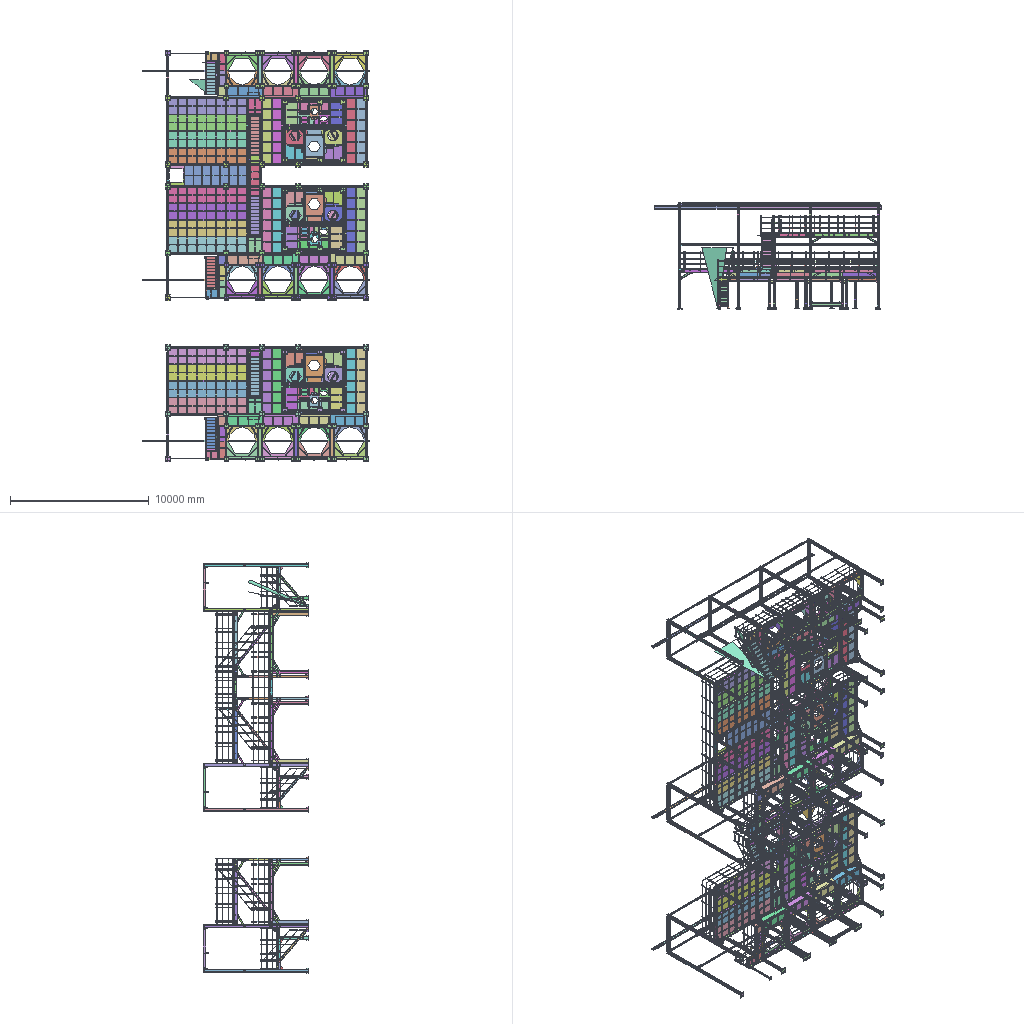Assembly | STEP file | 1060 different items | 5932 placed | box 16340 x 7600 x 29659 mm
Parts list (item | name | quantity | parent item | size | volume), first 203 of 1060 items:
1 | 粉仓立柱1主体_Default<As Machined> | x1 | in 粉仓立柱1 | 150 x 5128 x 194 mm | 19525526 mm3
2 | 立柱底Plate-400×350 | x10 | in 粉仓立柱1, 粉仓立柱2, 粉仓立柱3, 粉仓立柱4, 粉仓立柱5, 粉仓立柱6, 电柜立柱1, 电柜立柱2, 电柜立柱3, Electrical cabinet column 4 | 350 x 12 x 400 mm | 1654365 mm3
3 | 立柱Pad-400×350 | x10 | in 粉仓立柱1, 粉仓立柱2, 粉仓立柱3, 粉仓立柱4, 粉仓立柱5, 粉仓立柱6, 电柜立柱1, 电柜立柱2, 电柜立柱3, Electrical cabinet column 4 | 400 x 10 x 350 mm | 1384795 mm3
4 | 立柱底部筋Plate-200 | x32 | in 粉仓立柱1, 粉仓立柱2, 粉仓立柱3, 粉仓立柱4, 粉仓立柱5, 粉仓立柱6, 计量立柱1, 计量立柱2, 计量立柱3, 计量立柱4, 计量立柱5, 电柜立柱1, 电柜立柱2, 电柜立柱3, Electrical cabinet column 4 | 95 x 200 x 10 mm | 122000 mm3
5 | 立柱填充筋Plate-194×150 | x104 | in 粉仓立柱1, 粉仓立柱2, 粉仓立柱3, 粉仓立柱4, 粉仓立柱5, 粉仓立柱6, 计量立柱1, 计量立柱2, 计量立柱3, 计量立柱4, 电柜立柱1, 电柜立柱2, 电柜立柱3, Electrical cabinet column 4 | 72 x 10 x 176 mm | 125030 mm3
6 | 立柱腹Plate筋Plate-194×150-200 | x20 | in 粉仓立柱1, 粉仓立柱2, 粉仓立柱3, 粉仓立柱4, 粉仓立柱5, 粉仓立柱6, 计量立柱1, 计量立柱2, 计量立柱3, 计量立柱4, 电柜立柱1, 电柜立柱2, 电柜立柱3, Electrical cabinet column 4 | 230 x 180 x 10 mm | 352777 mm3
7 | 立柱翼Plate筋Plate-200 | x8 | in 粉仓立柱1, 粉仓立柱3, 粉仓立柱4, 粉仓立柱6, 电柜立柱1, 电柜立柱2, 电柜立柱3, Electrical cabinet column 4 | 155 x 150 x 10 mm | 203838 mm3
8 | 立柱填充筋Plate-194×150-1 | x2 | in 粉仓立柱1 | 72 x 10 x 176 mm | 115559 mm3
9 | 粉仓立柱2主体_Default<As Machined> | x1 | in 粉仓立柱2 | 150 x 5378 x 194 mm | 20480381 mm3
10 | 立柱腹Plate筋Plate-194×150-250 | x7 | in 粉仓立柱2, 粉仓立柱3, 粉仓立柱4, 粉仓立柱5, 粉仓立柱6 | 245 x 230 x 10 mm | 499277 mm3
11 | 立柱翼Plate筋Plate-250 | x9 | in 粉仓立柱2, 粉仓立柱3, 粉仓立柱4, 粉仓立柱5, 粉仓立柱6, 计量立柱1, 计量立柱2, 计量立柱3, 计量立柱4 | 155 x 210 x 10 mm | 296838 mm3
12 | 粉仓立柱3主体_Default<As Machined> | x1 | in 粉仓立柱3 | 150 x 5378 x 194 mm | 20474019 mm3
13 | Powder bin column 4 body_Default<As Machined> | x1 | in 粉仓立柱4 | 150 x 5378 x 194 mm | 20482501 mm3
14 | 立柱腹Plate筋Plate-194×150-12 | x10 | in 粉仓立柱4, 粉仓立柱5, 粉仓立柱6, 电柜立柱1, 电柜立柱2 | 200 x 100 x 8 mm | 126933 mm3
15 | Powder bin column 5 body_Default<As Machined> | x1 | in 粉仓立柱5 | 150 x 7578 x 194 mm | 28858083 mm3
16 | 立柱翼Plate筋Plate-150 | x4 | in 粉仓立柱5, 粉仓立柱6, 电柜立柱1, 电柜立柱2 | 154 x 154 x 10 mm | 217969 mm3
17 | 粉仓立柱6主体_Default<As Machined> | x1 | in 粉仓立柱6 | 150 x 7578 x 194 mm | 28847525 mm3
18 | 粉仓主梁1主体_Default<As Machined> | x1 | in 粉仓主梁1 | 4730 x 250 x 295 mm | 19829494 mm3
19 | Beam填充筋Plate-250×125 | x23 | in 粉仓主梁1, 粉仓主梁2, 粉仓主梁4, 粉仓主梁5, Powder bin main beam 7, 粉仓主梁8, 粉仓主梁9, 粉仓主梁11, 计量主梁1, 计量主梁2, 计量主梁5, 计量主梁6 | 55 x 10 x 232 mm | 126600 mm3
20 | 筋Plate-250×125-250 | x13 | in 粉仓主梁1, 粉仓主梁2, 粉仓主梁4, 粉仓主梁5, 粉仓主梁6, Powder bin main beam 7, 粉仓主梁11, 计量主梁1, 计量主梁2 | 215 x 232 x 10 mm | 429336 mm3
21 | 护栏连接Plate-250×125 | x29 | in 粉仓主梁1, 粉仓主梁2, 粉仓主梁3, 粉仓主梁4, Powder bin main beam 7, 粉仓主梁11 | 40 x 232 x 6 mm | 52883 mm3
22 | 筋Plate-250×125-200 | x10 | in 粉仓主梁1, 粉仓主梁5, 粉仓主梁6, Powder bin main beam 7, 粉仓主梁8, 粉仓主梁9, 粉仓主梁11, 计量主梁5 | 217 x 232 x 10 mm | 354786 mm3
23 | 筋Plate-250×125-150 | x30 | in 粉仓主梁1, 粉仓主梁2, 粉仓主梁3, 粉仓主梁4, 粉仓主梁5, 粉仓主梁6, 粉仓主梁8, 粉仓主梁9, 粉仓主梁10, 粉仓主梁11, 计量主梁1, 计量主梁2, 计量主梁6 | 190 x 232 x 10 mm | 269336 mm3
24 | 粉仓主梁2主体_Default<As Machined> | x1 | in 粉仓主梁2 | 4730 x 250 x 125 mm | 17453380 mm3
25 | 粉仓主梁3主体_Default<As Machined> | x1 | in 粉仓主梁3 | 2430 x 250 x 125 mm | 8963145 mm3
26 | 粉仓主梁4主体_Default<As Machined> | x1 | in 粉仓主梁4 | 4620 x 250 x 125 mm | 17048565 mm3
27 | 筋Plate-250×125-100 | x10 | in 粉仓主梁4, 粉仓主梁5, Powder bin main beam 7, 计量主梁1, 计量主梁2 | 185 x 232 x 8 mm | 168205 mm3
28 | Powder bin main beam 5 body_Default<As Machined> | x1 | in 粉仓主梁5 | 4586 x 250 x 125 mm | 16921020 mm3
29 | 筋Plate-250×125-150-30度 | x2 | in 粉仓主梁5, 粉仓主梁6 | 250 x 232 x 10 mm | 378866 mm3
30 | 筋Plate-250×125-200-30度 | x4 | in 粉仓主梁5, 粉仓主梁6, Powder bin main beam 7 | 265 x 232 x 10 mm | 450796 mm3
31 | 粉仓主梁6主体_Default<As Machined> | x1 | in 粉仓主梁6 | 4655 x 250 x 125 mm | 17188833 mm3
32 | 粉仓主梁7主体_Default<As Machined> | x1 | in Powder bin main beam 7 | 4586 x 250 x 125 mm | 16921020 mm3
33 | 粉仓主梁8主体_Default<As Machined> | x1 | in 粉仓主梁8 | 2455 x 250 x 125 mm | 9055569 mm3
34 | 筋Plate-250×125-200-60度 | x6 | in 粉仓主梁8, 粉仓主梁9, 粉仓主梁10 | 225 x 232 x 10 mm | 372036 mm3
35 | 粉仓主梁9主体_Default<As Machined> | x1 | in 粉仓主梁9 | 2655 x 250 x 125 mm | 9794957 mm3
36 | 粉仓主梁10主体_Default<As Machined> | x1 | in 粉仓主梁10 | 1955 x 250 x 125 mm | 7207100 mm3
37 | Powder bin main beam 11 body_Default<As Machined> | x1 | in 粉仓主梁11 | 3440 x 250 x 125 mm | 12683851 mm3
38 | 粉仓楼梯支撑Plate | x2 | in 粉仓主梁11 | 120 x 232 x 10 mm | 268929 mm3
39 | 护栏连接Plate-250×125-1 | x1 | in 粉仓主梁11 | 40 x 184 x 59.5 mm | 52864 mm3
40 | 粉仓主梁12主体_Default<As Machined> | x1 | in 粉仓主梁12 | 1815 x 200 x 360 mm | 5338714 mm3
41 | Beam填充筋Plate-200×100 | x7 | in 粉仓主梁12, 粉仓主梁13, 粉仓主梁14, 休息台主梁1, 休息台主梁2, 休息台主梁4, 休息台主梁5 | 8 x 184 x 37.25 mm | 54032 mm3
42 | 粉仓主梁13主体_Default<As Machined> | x1 | in 粉仓主梁13 | 2255 x 200 x 100 mm | 5995232 mm3
43 | 筋Plate-200×100-200 | x7 | in 粉仓主梁13, 休息台主梁1, 休息台主梁2, 休息台主梁4, 休息台主梁5, 计量主梁3 | 202 x 184 x 10 mm | 304236 mm3
44 | 筋Plate-200×100-150 | x16 | in 粉仓主梁13, 粉仓主梁15, 计量主梁4, 计量主梁7, 计量主梁8, 电柜主梁1, 电柜主梁3, 电柜主梁6 | 182 x 184 x 10 mm | 220956 mm3
45 | 筋Plate-200×100-200-30度 | x2 | in 粉仓主梁13, 粉仓主梁15 | 245 x 184 x 10 mm | 379966 mm3
46 | 粉仓主梁14主体_Default<As Machined> | x1 | in 粉仓主梁14 | 1955 x 200 x 360 mm | 5712085 mm3
47 | 粉仓主梁15主体_Default<As Machined> | x1 | in 粉仓主梁15 | 2255 x 200 x 100 mm | 5995232 mm3
48 | 粉仓辅梁1_Default<As Machined> | x1 | in 125Z正极线_粉仓Flat(E1) | 520 x 150 x 75 mm | 916827 mm3
49 | Powder bin secondary beam 2_Default<As Machined> | x1 | in 125Z正极线_粉仓Flat(E1) | 365 x 150 x 75 mm | 640161 mm3
50 | 粉仓辅梁3主体_Default<As Machined> | x2 | in 粉仓辅梁3 | 775 x 100 x 50 mm | 912656 mm3
51 | 粉仓辅梁4主体_Default<As Machined> | x1 | in 粉仓辅梁4 | 75 x 150 x 310 mm | 510249 mm3
52 | 粉仓辅梁5_Default<As Machined> | x1 | in 125Z正极线_粉仓Flat(E1) | 440 x 150 x 75 mm | 774032 mm3
53 | Powder bin secondary beam 6 body_Default<As Machined> | x1 | in 粉仓辅梁6 | 1245 x 150 x 350 mm | 2721156 mm3
54 | 粉仓辅梁7主体_Default<As Machined> | x1 | in 粉仓辅梁7 | 1545 x 150 x 280 mm | 3131691 mm3
55 | 粉仓辅梁8_Default<As Machined> | x1 | in 125Z正极线_粉仓Flat(E1) | 440 x 150 x 75 mm | 774032 mm3
56 | Powder bin secondary beam 9 body_Default<As Machined> | x1 | in 粉仓辅梁9 | 1445 x 150 x 75 mm | 2567894 mm3
57 | 筋Plate-150×75-150 | x18 | in 粉仓辅梁9, 粉仓辅梁10, 粉仓辅梁11, 粉仓辅梁13, 粉仓辅梁14, Powder bin secondary beam 16, 粉仓辅梁18, Metering secondary beam 5, Metering secondary beam 7, 计量辅梁15, Metering secondary beam 16 | 165 x 136 x 10 mm | 178316 mm3
58 | 筋Plate-150×75-150-60度 | x6 | in 粉仓辅梁9, 粉仓辅梁11, 粉仓辅梁14 | 175 x 136 x 10 mm | 189716 mm3
59 | 粉仓辅梁10主体_Default<As Machined> | x1 | in 粉仓辅梁10 | 2255 x 150 x 75 mm | 4013694 mm3
60 | 筋Plate-150×75-100 | x12 | in 粉仓辅梁10, 粉仓辅梁13, 粉仓辅梁18, 计量辅梁1, Metering secondary beam 5, 计量辅梁12, Metering secondary beam 16 | 165 x 136 x 8 mm | 100309 mm3
61 | 筋Plate-150×75-150-30度 | x4 | in 粉仓辅梁10, 粉仓辅梁13, Powder bin secondary beam 16, 粉仓辅梁18 | 200 x 136 x 10 mm | 222316 mm3
62 | 粉仓辅梁11主体_Default<As Machined> | x1 | in 粉仓辅梁11 | 1545 x 150 x 75 mm | 2746388 mm3
63 | 粉仓辅梁12_Default<As Machined> | x1 | in 125Z正极线_粉仓Flat(E1) | 430 x 150 x 75 mm | 756182 mm3
64 | 粉仓辅梁13主体_Default<As Machined> | x1 | in 粉仓辅梁13 | 2255 x 150 x 75 mm | 4013694 mm3
65 | 粉仓辅梁14主体_Default<As Machined> | x1 | in 粉仓辅梁14 | 1245 x 150 x 75 mm | 2210907 mm3
66 | 粉仓辅梁15主体_Default<As Machined> | x2 | in 粉仓辅梁15 | 915 x 100 x 50 mm | 1078548 mm3
67 | 粉仓辅梁16主体_Default<As Machined> | x1 | in Powder bin secondary beam 16 | 2255 x 150 x 230 mm | 4605807 mm3
68 | Powder bin secondary beam 17 body_Default<As Machined> | x2 | in 粉仓辅梁17 | 615 x 100 x 50 mm | 723066 mm3
69 | 粉仓辅梁18主体_Default<As Machined> | x1 | in 粉仓辅梁18 | 2255 x 150 x 75 mm | 4013694 mm3
70 | Powder bin diagonal beam 1_Default<As Machined> | x1 | in 125Z正极线_粉仓Flat(E1) | 502.735 x 200 x 870.763 mm | 2354862 mm3
71 | 粉仓Diagonal Brace梁2_Default<As Machined> | x1 | in 125Z正极线_粉仓Flat(E1) | 957.365 x 200 x 552.735 mm | 2621556 mm3
72 | 粉仓Diagonal Brace梁3-2_Default<As Machined> | x1 | in 125Z正极线_粉仓Flat(E1) | 253.301 x 150 x 438.731 mm | 738333 mm3
73 | 粉仓Diagonal Brace梁3-1_Default<As Machined> | x1 | in 125Z正极线_粉仓Flat(E1) | 273.301 x 150 x 473.372 mm | 809730 mm3
74 | 粉仓Diagonal Brace梁4_Default<As Machined> | x1 | in 125Z正极线_粉仓Flat(E1) | 473.372 x 150 x 273.301 mm | 809730 mm3
75 | Powder bin diagonal beam 5_Default<As Machined> | x1 | in 125Z正极线_粉仓Flat(E1) | 453.301 x 150 x 785.141 mm | 1452308 mm3
76 | 粉仓Diagonal Brace梁6-1_Default<As Machined> | x1 | in 125Z正极线_粉仓Flat(E1) | 525.333 x 150 x 303.301 mm | 916827 mm3
77 | 粉仓Diagonal Brace梁6-2_Default<As Machined> | x1 | in 125Z正极线_粉仓Flat(E1) | 646.577 x 150 x 373.301 mm | 1166718 mm3
78 | 粉仓Diagonal Brace梁7_Default<As Machined> | x1 | in 125Z正极线_粉仓Flat(E1) | 462.735 x 200 x 801.481 mm | 2141507 mm3
79 | 粉仓Diagonal Brace梁8_Default<As Machined> | x1 | in 125Z正极线_粉仓Flat(E1) | 671.577 x 200 x 387.735 mm | 1741466 mm3
80 | 粉仓Diagonal Brace梁9_Default<As Machined> | x1 | in 125Z正极线_粉仓Flat(E1) | 522.735 x 200 x 905.404 mm | 2461540 mm3
81 | 粉仓Diagonal Brace梁10_Default<As Machined> | x1 | in 125Z正极线_粉仓Flat(E1) | 1148 x 200 x 662.735 mm | 3208282 mm3
82 | 粉仓花纹Plate | x1 | in 125Z正极线_粉仓Flat(E1) | 7625 x 4925 x 3 mm | 81712704 mm3
83 | 休息台主梁1主体_Default<As Machined> | x1 | in 休息台主梁1 | 2430 x 200 x 200 mm | 6806772 mm3
84 | 筋Plate-200×100-5 | x34 | in 休息台主梁1, 休息台主梁2, 休息台主梁4, 休息台主梁5, Landing main beam 6, 计量主梁7, 计量主梁8, 电柜主梁2, 电柜主梁5, 电柜主梁8, 粉仓楼梯通道主梁1, 粉仓楼梯通道主梁2, 电柜通道主梁1 | 120 x 184 x 6 mm | 69909 mm3
85 | 护栏连接Plate-200×100 | x49 | in 休息台主梁1, 休息台主梁2, 休息台主梁3, 休息台主梁4, 休息台主梁5, Landing main beam 6, 电柜主梁2, 电柜主梁3, 电柜主梁4, 电柜主梁8, 粉仓楼梯通道主梁1, 粉仓楼梯通道主梁2, 电柜通道主梁1, Electrical cabinet walkway main beam 2 | 40 x 184 x 6 mm | 41363 mm3
86 | 休息台主梁2主体_Default<As Machined> | x1 | in 休息台主梁2 | 4730 x 200 x 200 mm | 13901578 mm3
87 | 休息台主梁3主体_Default<As Machined> | x1 | in 休息台主梁3 | 4586 x 200 x 100 mm | 12200555 mm3
88 | 筋Plate-200×100-100 | x50 | in 休息台主梁3, Landing main beam 6, Landing main beam 7, 休息台主梁8, 计量主梁3, 电柜主梁1, 电柜主梁3, 电柜主梁4, 电柜主梁6, 电柜主梁7, 电柜主梁9 | 182 x 184 x 8 mm | 124941 mm3
89 | Landing main beam 4 body_Default<As Machined> | x1 | in 休息台主梁4 | 4730 x 200 x 200 mm | 13878197 mm3
90 | 休息台主梁5主体_Default<As Machined> | x1 | in 休息台主梁5 | 2430 x 200 x 200 mm | 6806772 mm3
91 | 休息台主梁6主体_Default<As Machined> | x1 | in Landing main beam 6 | 4586 x 200 x 100 mm | 12200555 mm3
92 | 筋Plate-200×100-194 | x2 | in Landing main beam 6, 电柜主梁8 | 202 x 184 x 10 mm | 304236 mm3
93 | 休息台主梁7主体_Default<As Machined> | x1 | in Landing main beam 7 | 4680 x 200 x 100 mm | 12462557 mm3
94 | Landing main beam 8 body_Default<As Machined> | x1 | in 休息台主梁8 | 4680 x 200 x 100 mm | 12462557 mm3
95 | 休息台辅梁1主体_Default<As Machined> | x10 | in Landing secondary beam 1 | 1350 x 100 x 50 mm | 1593996 mm3
96 | 筋Plate-100×50-5 | x91 | in Landing secondary beam 1, 计量辅梁3, 计量辅梁11, 电柜辅梁1, 电柜辅梁3, 电柜通道辅梁1 | 95 x 86 x 6 mm | 27288 mm3
97 | 休息台角钢1_Default<As Machined> | x12 | in 125Z正极线_粉仓Flat(E1) | 721.5 x 50 x 50 mm | 278924 mm3
98 | 休息台花纹Plate 1 | x1 | in 125Z正极线_粉仓Flat(E1) | 1620 x 4900 x 3 mm | 23686830 mm3
99 | 休息台花纹Plate 2 | x1 | in 125Z正极线_粉仓Flat(E1) | 1620 x 4900 x 3 mm | 23500005 mm3
100 | 休息台花纹Plate 3 | x1 | in 125Z正极线_粉仓Flat(E1) | 4350 x 248 x 3 mm | 3156330 mm3
101 | 休息台花纹Plate 4 | x1 | in 125Z正极线_粉仓Flat(E1) | 4350 x 248 x 3 mm | 3156330 mm3
102 | Powder bin stair body_Default<As Machined> | x1 | in 粉仓楼梯 | 800 x 2588 x 3603 mm | 21206724 mm3
103 | 粉仓楼梯踏Plate 1 | x12 | in 粉仓楼梯 | 248 x 100 x 674 mm | 693251 mm3
104 | Stair base plate 2-1 | x2 | in 粉仓楼梯 | 120 x 160 x 12 mm | 218038 mm3
105 | 楼梯踏Plate 3 | x1 | in 粉仓楼梯 | 686 x 50 x 860 mm | 1690832 mm3
106 | Powder bin stair closing plate 1 | x12 | in 粉仓楼梯 | 674 x 3 x 100 mm | 202200 mm3
107 | 粉仓楼梯封Plate 2 | x1 | in 粉仓楼梯 | 674 x 3 x 138 mm | 279036 mm3
108 | 粉仓楼梯护栏1主体_Default<As Machined> | x2 | in 粉仓楼梯护栏1, 粉仓楼梯护栏2 | 25 x 3380 x 2914 mm | 1521542 mm3
109 | 楼梯护栏连接Plate 1 | x22 | in 粉仓楼梯护栏1, 粉仓楼梯护栏2, 中转釜楼梯护栏1, 中转釜楼梯护栏2 | 125 x 8 x 42 mm | 38206 mm3
110 | 粉仓护栏FixedPlate 1 | x2 | in 粉仓楼梯护栏2 | 85 x 40 x 40 mm | 13802 mm3
111 | Stair connecting plate 1 | x4 | in 粉仓楼梯, Transfer kettle stair | - | 160302 mm3
112 | 粉仓楼梯护栏连接Plate | x1 | in 粉仓楼梯 | 40 x 190.865 x 6 mm | 38885 mm3
113 | 粉仓护栏FixedPlate 2 | x2 | in 粉仓楼梯 | 45 x 40 x 63 mm | 11762 mm3
114 | 粉仓楼梯支承梁主体-194×150_Default<As Machined> | x1 | in 粉仓楼梯支承梁 | 940 x 150 x 194 mm | 3552325 mm3
115 | 筋Plate-194×150-100 | x1 | in 粉仓楼梯支承梁 | 200 x 176 x 8 mm | 160789 mm3
116 | 护栏90度栏杆_Default<As Machined> | x6 | in 护栏90度 | 397.5 x 25 x 397.5 mm | 82894 mm3
117 | 护栏90度立柱主体_Default<As Machined> | x4 | in 护栏90度立柱 | 40 x 1500 x 40 mm | 436819 mm3
118 | 40方管堵头 | x212 | in 护栏90度立柱, Powder bin guardrail 1 column, 护栏立柱2, 粉仓护栏2-1立柱, 粉仓护栏3-1立柱, 粉仓护栏3-2立柱, 粉仓护栏5立柱, 粉仓护栏立柱6, 粉仓护栏6-1立柱, 护栏立柱1, 粉仓护栏8-1立柱, 粉仓护栏8-2立柱, 粉仓护栏9立柱, Powder bin guardrail 9-1 column, 电柜护栏2立柱, 电柜护栏4立柱, 中转釜护栏2立柱, 中转釜护栏3立柱, 中转釜护栏4立柱, 中转釜护栏5立柱, 中转釜护栏7-1立柱, 中转釜护栏立柱7-2, Guardrail column 8-1, Guardrail column 8-2, Powder bin stair walkway guardrail 1 column, 粉仓楼梯通道护栏立柱2-1, 电柜通道护栏1立柱 | 40 x 18.9 x 40 mm | 8663 mm3
119 | 护栏90度踢脚Plate-1 | x2 | in 护栏90度 | 410 x 100 x 20 mm | 90870 mm3
120 | 护栏90度踢脚Plate-2 | x2 | in 护栏90度 | 410 x 100 x 20 mm | 119752 mm3
121 | 粉仓护栏1立柱主体_Default<As Machined> | x1 | in Powder bin guardrail 1 column | 40 x 1500 x 40 mm | 436819 mm3
122 | 护栏立柱2主体_Default<As Machined> | x60 | in 护栏立柱2 | 40 x 1500 x 40 mm | 432313 mm3
123 | 粉仓踢脚Plate 1 | x1 | in 粉仓护栏1 | 4345 x 100 x 20 mm | 998785 mm3
124 | 粉仓护栏栏杆1_Default<As Machined> | x1 | in 粉仓护栏1 | 4305 x 825 x 25 mm | 1430222 mm3
125 | 粉仓护栏2-1立柱主体_Default<As Machined> | x2 | in 粉仓护栏2-1立柱 | 40 x 1500 x 40 mm | 436819 mm3
126 | 粉仓踢脚Plate 2 | x1 | in 粉仓护栏2 | 3814 x 100 x 20 mm | 876724 mm3
127 | 粉仓护栏栏杆2_Default<As Machined> | x3 | in 粉仓护栏2 | 3734 x 25 x 25 mm | 413507 mm3
128 | Powder bin guardrail 3-1 column body_Default<As Machined> | x1 | in 粉仓护栏3-1立柱 | 40 x 1500 x 40 mm | 436819 mm3
129 | Powder bin toe plate 3 | x1 | in 粉仓护栏3 | 3694 x 100 x 20 mm | 849140 mm3
130 | 粉仓护栏栏杆3_Default<As Machined> | x1 | in 粉仓护栏3 | 3614 x 825 x 25 mm | 1200655 mm3
131 | 粉仓护栏3-2立柱主体_Default<As Machined> | x1 | in 粉仓护栏3-2立柱 | 40 x 1500 x 40 mm | 436531 mm3
132 | Powder bin toe plate 4 | x2 | in 粉仓护栏4 | 2430 x 100 x 20 mm | 558584 mm3
133 | 粉仓护栏栏杆4_Default<As Machined> | x2 | in 粉仓护栏4 | 2430 x 825 x 25 mm | 807303 mm3
134 | 粉仓踢脚Plate 5 | x1 | in 粉仓护栏5 | 2168 x 100 x 20 mm | 498243 mm3
135 | Powder bin guardrail rail 5_Default<As Machined> | x1 | in 粉仓护栏5 | 2128 x 825 x 25 mm | 706805 mm3
136 | 粉仓护栏5立柱主体_Default<As Machined> | x1 | in 粉仓护栏5立柱 | 40 x 1500 x 40 mm | 436819 mm3
137 | 粉仓踢脚Plate 6 | x1 | in 粉仓护栏6 | 2290 x 100 x 20 mm | 526402 mm3
138 | 粉仓护栏栏杆6_Default<As Machined> | x1 | in 粉仓护栏6 | 2250 x 825 x 25 mm | 747503 mm3
139 | 粉仓护栏6立柱主体_Default<As Machined> | x1 | in 粉仓护栏立柱6 | 40 x 1500 x 40 mm | 436819 mm3
140 | 粉仓踢脚Plate 6-1 | x1 | in 粉仓护栏6-1 | 2290 x 100 x 20 mm | 526402 mm3
141 | Powder bin guardrail rail 6-1_Default<As Machined> | x1 | in 粉仓护栏6-1 | 2250 x 825 x 25 mm | 747503 mm3
142 | 粉仓护栏6-1立柱主体_Default<As Machined> | x1 | in 粉仓护栏6-1立柱 | 40 x 1500 x 40 mm | 436819 mm3
143 | 护栏立柱1主体_Default<As Machined> | x9 | in 护栏立柱1 | 40 x 1500 x 40 mm | 438684 mm3
144 | Powder bin toe plate 7 | x1 | in Powder bin guardrail 7 | 3390 x 100 x 20 mm | 779259 mm3
145 | 粉仓护栏栏杆7_Default<As Machined> | x1 | in Powder bin guardrail 7 | 3350 x 825 x 25 mm | 1112948 mm3
146 | Powder bin guardrail 8-1 column body_Default<As Machined> | x1 | in 粉仓护栏8-1立柱 | 40 x 1500 x 40 mm | 436819 mm3
147 | 粉仓踢脚Plate 8 | x1 | in 粉仓护栏8 | 3330 x 100 x 20 mm | 765467 mm3
148 | 粉仓护栏栏杆8_Default<As Machined> | x3 | in 粉仓护栏8 | 3275 x 25 x 25 mm | 362677 mm3
149 | Powder bin guardrail 8-2 column body_Default<As Machined> | x1 | in 粉仓护栏8-2立柱 | 40 x 1500 x 40 mm | 436819 mm3
150 | 粉仓护栏9立柱主体_Default<As Machined> | x3 | in 粉仓护栏9立柱 | 40 x 1500 x 40 mm | 436819 mm3
151 | 粉仓踢脚Plate 9 | x3 | in 粉仓护栏9 | 2365 x 100 x 20 mm | 543643 mm3
152 | 粉仓护栏栏杆9_Default<As Machined> | x3 | in 粉仓护栏9 | 2325 x 825 x 25 mm | 772419 mm3
153 | 粉仓护栏9-1立柱主体_Default<As Machined> | x3 | in Powder bin guardrail 9-1 column | 40 x 1500 x 40 mm | 436819 mm3
154 | 粉仓踢脚Plate 9-1 | x3 | in 粉仓护栏9-1 | 2365 x 100 x 20 mm | 543643 mm3
155 | 粉仓护栏栏杆9-1_Default<As Machined> | x3 | in 粉仓护栏9-1 | 2325 x 825 x 25 mm | 772419 mm3
156 | Diagonal Brace矩形管-100×50-45度_Default<As Machined> | x1 | in Diagonal BraceComponent-45度 | 721.249 x 721.249 x 50 mm | 994577 mm3
157 | Diagonal Brace连接Plate-45度 | x2 | in Diagonal BraceComponent-45度 | 280 x 10 x 120 mm | 322431 mm3
158 | Diagonal Brace矩形管-60度_Default<As Machined> | x30 | in Diagonal BraceComponent-60度 | 823.131 x 475.235 x 50 mm | 902687 mm3
159 | Diagonal Brace连接Plate 1-1 | x30 | in Diagonal BraceComponent-60度 | 280 x 10 x 120 mm | 322431 mm3
160 | Diagonal Brace连接Plate 2-2 | x30 | in Diagonal BraceComponent-60度 | 360 x 10 x 100 mm | 346431 mm3
161 | 立柱底Plate-400×350-1 | x6 | in 计量立柱1, 计量立柱2, 计量立柱3, 计量立柱4, 计量立柱5 | - | -
162 | 立柱Pad-400×350-1 | x6 | in 计量立柱1, 计量立柱2, 计量立柱3, 计量立柱4, 计量立柱5 | 400 x 10 x 350 mm | 1384795 mm3
163 | 计量立柱1主体_Default<As Machined> | x1 | in 计量立柱1 | 150 x 2778 x 194 mm | 10580424 mm3
164 | Metering column 2 body_Default<As Machined> | x1 | in 计量立柱2 | 150 x 2778 x 194 mm | 10580424 mm3
165 | 计量立柱3主体_Default<As Machined> | x1 | in 计量立柱3 | 150 x 2778 x 194 mm | 10580424 mm3
166 | 计量立柱4主体_Default<As Machined> | x1 | in 计量立柱4 | 150 x 2778 x 194 mm | 10580424 mm3
167 | Metering column 5 body_Default<As Machined> | x2 | in 计量立柱5 | 150 x 2578 x 194 mm | 9824598 mm3
168 | 立柱填充筋Plate-194×150-2 | x4 | in 计量立柱5 | 72 x 10 x 176 mm | 115559 mm3
169 | 计量主梁1主体_Default<As Machined> | x1 | in 计量主梁1 | 3986 x 250 x 125 mm | 14702858 mm3
170 | 筋Plate-250×125-150-45度 | x6 | in 计量主梁1, 计量主梁2, 计量主梁5 | 215 x 232 x 10 mm | 315156 mm3
171 | 计量主梁2主体_Default<As Machined> | x1 | in 计量主梁2 | 3986 x 250 x 125 mm | 14702858 mm3
172 | 计量主梁3主体_Default<As Machined> | x1 | in 计量主梁3 | 4030 x 200 x 100 mm | 10713895 mm3
173 | Beam填充筋Plate-200×100-2 | x4 | in 计量主梁3, 计量主梁4 | 45 x 10 x 184 mm | 81800 mm3
174 | 计量主梁主4体_Default<As Machined> | x1 | in 计量主梁4 | 4030 x 200 x 100 mm | 10713895 mm3
175 | 计量主梁5主体_Default<As Machined> | x1 | in 计量主梁5 | 4055 x 250 x 125 mm | 14970670 mm3
176 | 计量主梁6主体_Default<As Machined> | x1 | in 计量主梁6 | 4055 x 250 x 125 mm | 14970670 mm3
177 | 筋Plate-250×125-5 | x1 | in 计量主梁6 | 135 x 232 x 6 mm | 105651 mm3
178 | 计量主梁7主体_Default<As Machined> | x1 | in 计量主梁7 | 2170 x 200 x 100 mm | 5768543 mm3
179 | 筋Plate-200×100-150 -45度 | x2 | in 计量主梁7, 计量主梁8 | 196 x 184 x 10 mm | 240506 mm3
180 | 计量主梁8主体_Default<As Machined> | x1 | in 计量主梁8 | 2170 x 200 x 100 mm | 5768543 mm3
181 | 计量辅梁1主体_Default<As Machined> | x1 | in 计量辅梁1 | 1268 x 150 x 75 mm | 2251068 mm3
182 | 计量辅梁2_Default<As Machined> | x1 | in 125Z正极线_计量Flat(E1) | 1280 x 150 x 75 mm | 2273380 mm3
183 | Metering secondary beam 3 body_Default<As Machined> | x1 | in 计量辅梁3 | 1015 x 100 x 50 mm | 1197042 mm3
184 | Metering secondary beam 4 body_Default<As Machined> | x1 | in 计量辅梁4 | 1280 x 150 x 75 mm | 2273380 mm3
185 | 计量辅梁5主体_Default<As Machined> | x1 | in Metering secondary beam 5 | 1540 x 150 x 75 mm | 2737463 mm3
186 | 筋Plate-150×75-5 | x17 | in Metering secondary beam 5, Metering secondary beam 7, 计量辅梁8, 计量辅梁15, Metering secondary beam 16, 电柜辅梁2 | 110 x 136 x 6 mm | 47835 mm3
187 | Metering secondary beam 6_Default<As Machined> | x1 | in 125Z正极线_计量Flat(E1) | 605 x 150 x 75 mm | 1068546 mm3
188 | 计量辅梁7主体_Default<As Machined> | x1 | in Metering secondary beam 7 | 1540 x 150 x 75 mm | 2737463 mm3
189 | 计量辅梁8主体_Default<As Machined> | x1 | in 计量辅梁8 | 600 x 150 x 75 mm | 1059622 mm3
190 | 计量辅梁9_Default<As Machined> | x1 | in 125Z正极线_计量Flat(E1) | 600 x 150 x 75 mm | 1059622 mm3
191 | 计量辅梁10主体_Default<As Machined> | x2 | in 计量辅梁10 | 932.5 x 100 x 50 mm | 1099284 mm3
192 | 计量辅梁11主体_Default<As Machined> | x1 | in 计量辅梁11 | 1015 x 100 x 50 mm | 1197042 mm3
193 | 计量辅梁12主体_Default<As Machined> | x1 | in 计量辅梁12 | 1268 x 150 x 75 mm | 2251068 mm3
194 | 计量辅梁13主体_Default<As Machined> | x2 | in 计量辅梁13 | 932.5 x 100 x 50 mm | 1099284 mm3
195 | 计量辅梁14_Default<As Machined> | x1 | in 125Z正极线_计量Flat(E1) | 605 x 150 x 75 mm | 1068546 mm3
196 | 计量辅梁15主体_Default<As Machined> | x1 | in 计量辅梁15 | 1540 x 150 x 75 mm | 2737463 mm3
197 | 计量辅梁16主体_Default<As Machined> | x1 | in Metering secondary beam 16 | 1540 x 150 x 75 mm | 2737463 mm3
198 | 计量Diagonal Brace梁1_Default<As Machined> | x1 | in 125Z正极线_计量Flat(E1) | 300.52 x 150 x 300.52 mm | 613387 mm3
199 | 计量Diagonal Brace梁2_Default<As Machined> | x1 | in 125Z正极线_计量Flat(E1) | 300.52 x 150 x 300.52 mm | 613387 mm3
200 | 计量Diagonal Brace梁3_Default<As Machined> | x1 | in 125Z正极线_计量Flat(E1) | 265.165 x 150 x 265.165 mm | 524140 mm3
201 | Metering diagonal beam 4_Default<As Machined> | x1 | in 125Z正极线_计量Flat(E1) | 265.165 x 150 x 265.165 mm | 524140 mm3
202 | 计量Pad 1 | x1 | in 125Z正极线_计量Flat(E1) | 2185 x 10 x 4350 mm | 56422097 mm3
203 | Metering pad plate 2 | x1 | in 125Z正极线_计量Flat(E1) | 1510 x 12 x 2370 mm | 24906794 mm3
Placements (level | parent | child | x y z in mm | rotation matrix by rows), first 206 of 6860 lines:
1 | 125Z正极线_钢结构主FlatMain Assembly | 125Z正极线_钢结构主Flat(E1+E2) | -3126.813 3252.909 7628.76 | 1 0 0 0 1 0 0 0 1
2 | 125Z正极线_钢结构主Flat(E1+E2) | 125Z正极线_钢结构主Flat(E1) | 6780.545 6742.472 1946.529 | 1 0 0 0 1 0 0 0 1
3 | 125Z正极线_钢结构主Flat(E1) | 125Z正极线_粉仓Flat(E1) | -1001.675 1556.727 -1180.753 | 1 0 0 0 1 0 0 0 1
4 | 125Z正极线_粉仓Flat(E1) | 粉仓立柱1 | 2972.354 691.954 2446.101 | 1 0 0 0 1 0 0 0 1
5 | 粉仓立柱1 | 粉仓立柱1主体_Default<As Machined> | -0.0 -0.0 -0.0 | 1 0 0 0 1 0 0 0 1
5 | 粉仓立柱1 | 立柱底Plate-400×350 | -0.0 -12.0 0.0 | -1 0 0 0 1 0 0 0 -1
5 | 粉仓立柱1 | 立柱Pad-400×350 | -0.0 -22.0 -0.0 | 0 0 1 0 1 0 -1 0 0
5 | 粉仓立柱1 | 立柱底部筋Plate-200 | -0.0 -0.0 97.0 | 0 0 -1 0 1 0 1 0 0
5 | 粉仓立柱1 | 立柱底部筋Plate-200 | -0.0 -0.0 -97.0 | 0 0 1 0 1 0 -1 0 0
5 | 粉仓立柱1 | 立柱填充筋Plate-194×150 | 3.0 2778.0 0.0 | 1 0 0 0 -1 0 0 0 -1
5 | 粉仓立柱1 | 立柱腹Plate筋Plate-194×150-200 | 118.0 2678.0 8.0 | 1 0 0 0 1 0 0 0 1
5 | 粉仓立柱1 | 立柱填充筋Plate-194×150 | 3.0 2588.0 0.0 | 1 0 0 0 -1 0 0 0 -1
5 | 粉仓立柱1 | 立柱翼Plate筋Plate-200 | 7.75 2683.0 174.5 | 0 0 -1 0 1 0 1 0 0
5 | 粉仓立柱1 | 立柱填充筋Plate-194×150 | -3.0 2778.0 0.0 | -1 0 0 0 -1 0 0 0 1
5 | 粉仓立柱1 | 立柱填充筋Plate-194×150 | -3.0 2588.0 0.0 | -1 0 0 0 -1 0 0 0 1
5 | 粉仓立柱1 | 立柱腹Plate筋Plate-194×150-200 | -118.0 2678.0 8.0 | -1 0 0 0 1 0 0 0 -1
5 | 粉仓立柱1 | 立柱填充筋Plate-194×150-1 | 3.0 5128.0 -0.0 | 1 0 0 0 -1 0 0 0 -1
5 | 粉仓立柱1 | 立柱填充筋Plate-194×150-1 | -3.0 5128.0 -0.0 | -1 0 0 0 -1 0 0 0 1
4 | 125Z正极线_粉仓Flat(E1) | 粉仓立柱2 | 5572.354 691.954 2446.101 | 1 0 0 0 1 0 0 0 1
5 | 粉仓立柱2 | 粉仓立柱2主体_Default<As Machined> | -0.0 -0.0 -0.0 | 1 0 0 0 1 0 0 0 1
5 | 粉仓立柱2 | 立柱底Plate-400×350 | -0.0 -12.0 0.0 | -1 0 0 0 1 0 0 0 -1
5 | 粉仓立柱2 | 立柱Pad-400×350 | -0.0 -22.0 -0.0 | 0 0 1 0 1 0 -1 0 0
5 | 粉仓立柱2 | 立柱底部筋Plate-200 | -0.0 -0.0 97.0 | 0 0 -1 0 1 0 1 0 0
5 | 粉仓立柱2 | 立柱填充筋Plate-194×150 | 3.0 5378.0 -0.0 | 1 0 0 0 -1 0 0 0 -1
5 | 粉仓立柱2 | 立柱填充筋Plate-194×150 | -3.0 5378.0 -0.0 | -1 0 0 0 -1 0 0 0 1
5 | 粉仓立柱2 | 立柱底部筋Plate-200 | -0.0 -0.0 -97.0 | 0 0 1 0 1 0 -1 0 0
5 | 粉仓立柱2 | 立柱填充筋Plate-194×150 | 3.0 2778.0 0.0 | 1 0 0 0 -1 0 0 0 -1
5 | 粉仓立柱2 | 立柱腹Plate筋Plate-194×150-200 | 118.0 2678.0 8.0 | 1 0 0 0 1 0 0 0 1
5 | 粉仓立柱2 | 立柱填充筋Plate-194×150 | 3.0 2588.0 0.0 | 1 0 0 0 -1 0 0 0 -1
5 | 粉仓立柱2 | 立柱填充筋Plate-194×150 | -3.0 2778.0 0.0 | -1 0 0 0 -1 0 0 0 1
5 | 粉仓立柱2 | 立柱填充筋Plate-194×150 | -3.0 2588.0 0.0 | -1 0 0 0 -1 0 0 0 1
5 | 粉仓立柱2 | 立柱腹Plate筋Plate-194×150-200 | -118.0 2678.0 8.0 | -1 0 0 0 1 0 0 0 -1
5 | 粉仓立柱2 | 立柱腹Plate筋Plate-194×150-250 | 125.5 5253.0 8.0 | 1 0 0 0 1 0 0 0 1
5 | 粉仓立柱2 | 立柱腹Plate筋Plate-194×150-250 | -125.5 5253.0 8.0 | -1 0 0 0 1 0 0 0 -1
5 | 粉仓立柱2 | 立柱填充筋Plate-194×150 | 3.0 5138.0 -0.0 | 1 0 0 0 -1 0 0 0 -1
5 | 粉仓立柱2 | 立柱填充筋Plate-194×150 | -3.0 5138.0 -0.0 | -1 0 0 0 -1 0 0 0 1
5 | 粉仓立柱2 | 立柱翼Plate筋Plate-250 | 8.0 5253.0 174.5 | 0 0 -1 0 1 0 1 0 0
4 | 125Z正极线_粉仓Flat(E1) | 粉仓立柱3 | 10472.354 691.954 2446.101 | 1 0 0 0 1 0 0 0 1
5 | 粉仓立柱3 | 粉仓立柱3主体_Default<As Machined> | -0.0 -0.0 -0.0 | 1 0 0 0 1 0 0 0 1
5 | 粉仓立柱3 | 立柱底Plate-400×350 | -0.0 -12.0 0.0 | -1 0 0 0 1 0 0 0 -1
5 | 粉仓立柱3 | 立柱Pad-400×350 | -0.0 -22.0 -0.0 | 0 0 1 0 1 0 -1 0 0
5 | 粉仓立柱3 | 立柱底部筋Plate-200 | -0.0 -0.0 97.0 | 0 0 -1 0 1 0 1 0 0
5 | 粉仓立柱3 | 立柱填充筋Plate-194×150 | 3.0 5378.0 -0.0 | 1 0 0 0 -1 0 0 0 -1
5 | 粉仓立柱3 | 立柱填充筋Plate-194×150 | -3.0 5378.0 -0.0 | -1 0 0 0 -1 0 0 0 1
5 | 粉仓立柱3 | 立柱底部筋Plate-200 | -0.0 -0.0 -97.0 | 0 0 1 0 1 0 -1 0 0
5 | 粉仓立柱3 | 立柱填充筋Plate-194×150 | -3.0 2778.0 0.0 | -1 0 0 0 -1 0 0 0 1
5 | 粉仓立柱3 | 立柱填充筋Plate-194×150 | -3.0 2588.0 0.0 | -1 0 0 0 -1 0 0 0 1
5 | 粉仓立柱3 | 立柱腹Plate筋Plate-194×150-200 | -118.0 2678.0 8.0 | -1 0 0 0 1 0 0 0 -1
5 | 粉仓立柱3 | 立柱翼Plate筋Plate-200 | -8.0 2683.0 174.5 | 0 0 -1 0 1 0 1 0 0
5 | 粉仓立柱3 | 立柱填充筋Plate-194×150 | 3.0 2778.0 0.0 | 1 0 0 0 -1 0 0 0 -1
5 | 粉仓立柱3 | 立柱填充筋Plate-194×150 | 3.0 2588.0 0.0 | 1 0 0 0 -1 0 0 0 -1
5 | 粉仓立柱3 | 立柱翼Plate筋Plate-250 | -8.0 5253.0 174.5 | 0 0 -1 0 1 0 1 0 -0
5 | 粉仓立柱3 | 立柱腹Plate筋Plate-194×150-250 | -125.5 5253.0 8.0 | -1 0 0 0 1 0 0 0 -1
5 | 粉仓立柱3 | 立柱填充筋Plate-194×150 | 3.0 5138.0 -0.0 | 1 0 0 0 -1 0 0 0 -1
5 | 粉仓立柱3 | 立柱填充筋Plate-194×150 | -3.0 5138.0 -0.0 | -1 0 0 0 -1 0 0 0 1
4 | 125Z正极线_粉仓Flat(E1) | 粉仓立柱4 | 2972.354 691.954 7246.1 | 1 0 0 0 1 0 0 0 1
5 | 粉仓立柱4 | Powder bin column 4 body_Default<As Machined> | -0.0 -0.0 -0.0 | 1 0 0 0 1 0 0 0 1
5 | 粉仓立柱4 | 立柱底Plate-400×350 | -0.0 -12.0 0.0 | -1 0 0 0 1 0 0 0 -1
5 | 粉仓立柱4 | 立柱Pad-400×350 | -0.0 -22.0 -0.0 | 0 0 1 0 1 0 -1 0 0
5 | 粉仓立柱4 | 立柱底部筋Plate-200 | -0.0 -0.0 97.0 | 0 0 -1 0 1 0 1 0 0
5 | 粉仓立柱4 | 立柱底部筋Plate-200 | -0.0 -0.0 -97.0 | 0 0 1 0 1 0 -1 0 0
5 | 粉仓立柱4 | 立柱填充筋Plate-194×150 | 3.0 2778.0 0.0 | 1 0 0 0 -1 0 0 0 -1
5 | 粉仓立柱4 | 立柱填充筋Plate-194×150 | -3.0 2778.0 0.0 | -1 0 0 0 -1 0 0 0 1
5 | 粉仓立柱4 | 立柱填充筋Plate-194×150 | -3.0 2588.0 0.0 | -1 0 0 0 -1 0 0 0 1
5 | 粉仓立柱4 | 立柱填充筋Plate-194×150 | 3.0 2588.0 0.0 | 1 0 0 0 -1 0 0 0 -1
5 | 粉仓立柱4 | 立柱腹Plate筋Plate-194×150-200 | 118.0 2678.0 -7.75 | 1 0 0 0 1 0 0 0 1
5 | 粉仓立柱4 | 立柱填充筋Plate-194×150 | 3.0 5378.0 -0.0 | 1 0 0 0 -1 0 0 0 -1
5 | 粉仓立柱4 | 立柱填充筋Plate-194×150 | 3.0 5138.0 -0.0 | 1 0 0 0 -1 0 0 0 -1
5 | 粉仓立柱4 | 立柱翼Plate筋Plate-250 | 7.75 5253.0 -174.5 | 0 0 1 0 1 0 -1 0 0
5 | 粉仓立柱4 | 立柱腹Plate筋Plate-194×150-250 | 125.5 5253.0 -7.75 | 1 0 0 0 1 0 0 0 1
5 | 粉仓立柱4 | 立柱翼Plate筋Plate-200 | 7.75 2683.0 -174.5 | 0 0 1 0 1 0 -1 0 -0
5 | 粉仓立柱4 | 立柱填充筋Plate-194×150 | -3.0 5378.0 -0.0 | -1 0 0 0 -1 0 0 0 1
5 | 粉仓立柱4 | 立柱腹Plate筋Plate-194×150-12 | -103.0 4618.0 -0.0 | -1 0 0 0 1 0 0 0 -1
5 | 粉仓立柱4 | 立柱填充筋Plate-194×150 | -3.0 5138.0 -0.0 | -1 0 0 0 -1 0 0 0 1
5 | 粉仓立柱4 | 立柱腹Plate筋Plate-194×150-200 | -118.0 2678.0 -7.75 | -1 0 0 0 1 0 0 0 -1
5 | 粉仓立柱4 | 立柱填充筋Plate-194×150 | -3.0 4678.0 0.0 | -1 0 0 0 -1 0 0 0 1
5 | 粉仓立柱4 | 立柱填充筋Plate-194×150 | -3.0 4568.0 0.0 | -1 0 0 0 -1 0 0 0 1
4 | 125Z正极线_粉仓Flat(E1) | 粉仓立柱5 | 5572.354 691.954 7246.1 | 1 0 0 0 1 0 0 0 1
5 | 粉仓立柱5 | Powder bin column 5 body_Default<As Machined> | -0.0 -0.0 -0.0 | 1 0 0 0 1 0 0 0 1
5 | 粉仓立柱5 | 立柱底Plate-400×350 | -0.0 -12.0 0.0 | -1 0 0 0 1 0 0 0 -1
5 | 粉仓立柱5 | 立柱Pad-400×350 | -0.0 -22.0 -0.0 | 0 0 1 0 1 0 -1 0 0
5 | 粉仓立柱5 | 立柱底部筋Plate-200 | 25.0 0.0 97.0 | 0 0 -1 0 1 0 1 0 0
5 | 粉仓立柱5 | 立柱填充筋Plate-194×150 | 3.0 7578.0 -0.0 | 1 0 0 0 -1 0 0 0 -1
5 | 粉仓立柱5 | 立柱填充筋Plate-194×150 | -3.0 7578.0 -0.0 | -1 0 0 0 -1 0 0 0 1
5 | 粉仓立柱5 | 立柱底部筋Plate-200 | 25.0 -0.0 -97.0 | 0 0 1 0 1 0 -1 0 0
5 | 粉仓立柱5 | 立柱填充筋Plate-194×150 | 3.0 2778.0 0.0 | 1 0 0 0 -1 0 0 0 -1
5 | 粉仓立柱5 | 立柱腹Plate筋Plate-194×150-250 | 125.5 5253.0 -8.0 | 1 0 0 0 1 0 0 0 1
5 | 粉仓立柱5 | 立柱腹Plate筋Plate-194×150-250 | -125.5 5253.0 -8.0 | -1 0 0 0 1 0 0 0 -1
5 | 粉仓立柱5 | 立柱填充筋Plate-194×150 | 3.0 2588.0 0.0 | 1 0 0 0 -1 0 0 0 -1
5 | 粉仓立柱5 | 立柱腹Plate筋Plate-194×150-200 | 118.0 2678.0 -7.75 | 1 0 0 0 1 0 0 0 1
5 | 粉仓立柱5 | 立柱填充筋Plate-194×150 | 3.0 5378.0 -0.0 | 1 0 0 0 -1 0 0 0 -1
5 | 粉仓立柱5 | 立柱填充筋Plate-194×150 | 3.0 5138.0 -0.0 | 1 0 0 0 -1 0 0 0 -1
5 | 粉仓立柱5 | 立柱填充筋Plate-194×150 | -3.0 5378.0 -0.0 | -1 0 0 0 -1 0 0 0 1
5 | 粉仓立柱5 | 立柱填充筋Plate-194×150 | -3.0 5138.0 -0.0 | -1 0 0 0 -1 0 0 0 1
5 | 粉仓立柱5 | 立柱填充筋Plate-194×150 | -3.0 2778.0 0.0 | -1 0 0 0 -1 0 0 0 1
5 | 粉仓立柱5 | 立柱腹Plate筋Plate-194×150-200 | -118.0 2678.0 -7.75 | -1 0 0 0 1 0 0 0 -1
5 | 粉仓立柱5 | 立柱填充筋Plate-194×150 | -3.0 2588.0 0.0 | -1 0 0 0 -1 0 0 0 1
5 | 粉仓立柱5 | 立柱腹Plate筋Plate-194×150-12 | -103.0 7518.0 -0.0 | -1 0 0 0 1 0 0 0 -1
5 | 粉仓立柱5 | 立柱填充筋Plate-194×150 | 3.0 7468.0 -0.0 | 1 0 0 0 -1 0 0 0 -1
5 | 粉仓立柱5 | 立柱填充筋Plate-194×150 | -3.0 7468.0 -0.0 | -1 0 0 0 -1 0 0 0 1
5 | 粉仓立柱5 | 立柱腹Plate筋Plate-194×150-12 | 103.0 7518.0 -0.0 | 1 0 0 0 1 0 0 0 1
5 | 粉仓立柱5 | 立柱翼Plate筋Plate-150 | 8.0 7481.0 174.0 | 0 0 -1 0 1 0 1 0 -0
5 | 粉仓立柱5 | 立柱翼Plate筋Plate-250 | -8.0 5253.0 -174.5 | 0 0 1 0 1 0 -1 0 0
4 | 125Z正极线_粉仓Flat(E1) | 粉仓立柱6 | 10472.354 691.954 7246.1 | 1 0 0 0 1 0 0 0 1
5 | 粉仓立柱6 | 粉仓立柱6主体_Default<As Machined> | -0.0 -0.0 -0.0 | 1 0 0 0 1 0 0 0 1
5 | 粉仓立柱6 | 立柱底Plate-400×350 | -0.0 -12.0 0.0 | -1 0 0 0 1 0 0 0 -1
5 | 粉仓立柱6 | 立柱Pad-400×350 | -0.0 -22.0 -0.0 | 0 0 1 0 1 0 -1 0 0
5 | 粉仓立柱6 | 立柱底部筋Plate-200 | -0.0 -0.0 97.0 | 0 0 -1 0 1 0 1 0 0
5 | 粉仓立柱6 | 立柱填充筋Plate-194×150 | 3.0 7578.0 -0.0 | 1 0 0 0 -1 0 0 0 -1
5 | 粉仓立柱6 | 立柱填充筋Plate-194×150 | -3.0 7578.0 -0.0 | -1 0 0 0 -1 0 0 0 1
5 | 粉仓立柱6 | 立柱底部筋Plate-200 | -0.0 -0.0 -97.0 | 0 0 1 0 1 0 -1 0 0
5 | 粉仓立柱6 | 立柱填充筋Plate-194×150 | -3.0 2778.0 0.0 | -1 0 0 0 -1 0 0 0 1
5 | 粉仓立柱6 | 立柱腹Plate筋Plate-194×150-250 | -125.5 5253.0 -8.0 | -1 0 0 0 1 0 0 0 -1
5 | 粉仓立柱6 | 立柱翼Plate筋Plate-250 | -8.0 5253.0 -174.5 | 0 0 1 0 1 0 -1 0 -0
5 | 粉仓立柱6 | 立柱填充筋Plate-194×150 | -3.0 2588.0 0.0 | -1 0 0 0 -1 0 0 0 1
5 | 粉仓立柱6 | 立柱填充筋Plate-194×150 | -3.0 5378.0 -0.0 | -1 0 0 0 -1 0 0 0 1
5 | 粉仓立柱6 | 立柱填充筋Plate-194×150 | -3.0 2778.0 0.0 | -1 0 0 0 -1 0 0 0 1
5 | 粉仓立柱6 | 立柱填充筋Plate-194×150 | -3.0 5138.0 -0.0 | -1 0 0 0 -1 0 0 0 1
5 | 粉仓立柱6 | 立柱腹Plate筋Plate-194×150-200 | -118.0 2678.0 -7.75 | -1 0 0 0 1 0 0 0 -1
5 | 粉仓立柱6 | 立柱翼Plate筋Plate-200 | -8.0 2683.0 -174.5 | 0 0 1 0 1 0 -1 0 0
5 | 粉仓立柱6 | 立柱填充筋Plate-194×150 | 3.0 7468.0 -0.0 | 1 0 0 0 -1 0 0 0 -1
5 | 粉仓立柱6 | 立柱填充筋Plate-194×150 | -3.0 7468.0 -0.0 | -1 0 0 0 -1 0 0 0 1
5 | 粉仓立柱6 | 立柱填充筋Plate-194×150 | 3.0 5378.0 -0.0 | 1 0 0 0 -1 0 0 0 -1
5 | 粉仓立柱6 | 立柱填充筋Plate-194×150 | 3.0 5138.0 -0.0 | 1 0 0 0 -1 0 0 0 -1
5 | 粉仓立柱6 | 立柱填充筋Plate-194×150 | 3.0 2588.0 0.0 | 1 0 0 0 -1 0 0 0 -1
5 | 粉仓立柱6 | 立柱腹Plate筋Plate-194×150-12 | -103.0 7518.0 -0.0 | -1 0 0 0 1 0 0 0 -1
5 | 粉仓立柱6 | 立柱翼Plate筋Plate-150 | -8.0 7481.0 174.0 | 0 0 -1 0 1 0 1 0 -0
5 | 粉仓立柱6 | 立柱填充筋Plate-194×150 | 3.0 2748.0 0.0 | 1 0 0 0 -1 0 0 0 -1
4 | 125Z正极线_粉仓Flat(E1) | 粉仓主梁1 | 10494.354 3381.954 2446.101 | -1 0 0 0 1 0 0 0 -1
5 | 粉仓主梁1 | 粉仓主梁1主体_Default<As Machined> | 107.0 2688.0 -0.0 | 1 0 0 0 1 0 0 0 1
5 | 粉仓主梁1 | Beam填充筋Plate-250×125 | 2119.5 2563.0 3.0 | 0 -1 0 0 0 -1 1 0 -0
5 | 粉仓主梁1 | Beam填充筋Plate-250×125 | 1084.5 2563.0 3.0 | 0 -1 0 0 0 -1 1 0 -0
5 | 粉仓主梁1 | 筋Plate-250×125-250 | 2114.5 2563.0 -110.5 | 0 0 1 0 1 0 -1 0 0
5 | 粉仓主梁1 | 护栏连接Plate-250×125 | 389.5 2587.0 62.5 | -1 0 0 0 1 0 0 0 -1
5 | 粉仓主梁1 | 护栏连接Plate-250×125 | 349.5 2587.0 62.5 | -1 0 0 0 1 0 0 0 -1
5 | 粉仓主梁1 | 护栏连接Plate-250×125 | 1649.5 2587.0 62.5 | -1 0 0 0 1 0 0 0 -1
5 | 粉仓主梁1 | 护栏连接Plate-250×125 | 2909.5 2587.0 62.5 | -1 0 0 0 1 0 0 0 -1
5 | 粉仓主梁1 | 护栏连接Plate-250×125 | 4169.5 2587.0 62.5 | -1 0 0 0 1 0 0 0 -1
5 | 粉仓主梁1 | 护栏连接Plate-250×125 | 4212.0 2587.0 62.5 | -1 0 0 0 1 0 0 0 -1
5 | 粉仓主梁1 | 筋Plate-250×125-200 | 4416.75 2563.0 -111.5 | 0 0 1 0 1 0 -1 0 -0
5 | 粉仓主梁1 | 筋Plate-250×125-150 | 1079.5 2563.0 -98.0 | 0 0 1 0 1 0 -1 0 0
5 | 粉仓主梁1 | Beam填充筋Plate-250×125 | 3036.75 2563.0 3.0 | 0 -1 0 0 0 -1 1 0 -0
5 | 粉仓主梁1 | Beam填充筋Plate-250×125 | 3532.25 2563.0 3.0 | 0 -1 0 0 0 -1 1 0 -0
5 | 粉仓主梁1 | Beam填充筋Plate-250×125 | 4421.75 2563.0 3.0 | 0 -1 0 0 0 -1 1 0 -0
4 | 125Z正极线_粉仓Flat(E1) | 粉仓主梁2 | 10494.354 3381.954 3246.101 | -1 0 0 0 1 0 0 0 -1
5 | 粉仓主梁2 | 粉仓主梁2主体_Default<As Machined> | 107.0 2688.0 -4000.0 | 1 0 0 0 1 0 0 0 1
5 | 粉仓主梁2 | 筋Plate-250×125-250 | 2130.0 2563.0 -3889.5 | 0 0 -1 0 1 0 1 0 -0
5 | 粉仓主梁2 | Beam填充筋Plate-250×125 | 2125.0 2563.0 -4003.0 | 0 1 0 0 0 -1 -1 0 0
5 | 粉仓主梁2 | 筋Plate-250×125-150 | 749.5 2563.0 -3902.0 | 0 0 -1 0 1 0 1 0 -0
5 | 粉仓主梁2 | 护栏连接Plate-250×125 | 4612.0 2587.0 -4056.5 | -1 0 0 0 1 0 0 0 -1
5 | 粉仓主梁2 | 护栏连接Plate-250×125 | 3552.0 2587.0 -4056.5 | -1 0 0 0 1 0 0 0 -1
5 | 粉仓主梁2 | 护栏连接Plate-250×125 | 2492.0 2587.0 -4056.5 | -1 0 0 0 1 0 0 0 -1
5 | 粉仓主梁2 | 护栏连接Plate-250×125 | 2452.0 2587.0 -4056.5 | -1 0 0 0 1 0 0 0 -1
5 | 粉仓主梁2 | 护栏连接Plate-250×125 | 1392.0 2587.0 -4056.5 | -1 0 0 0 1 0 0 0 -1
5 | 粉仓主梁2 | 护栏连接Plate-250×125 | 332.0 2587.0 -4056.5 | -1 0 0 0 1 0 0 0 -1
5 | 粉仓主梁2 | 筋Plate-250×125-150 | 1419.5 2563.0 -3902.0 | 0 0 -1 0 1 0 1 0 -0
5 | 粉仓主梁2 | 筋Plate-250×125-150 | 2379.5 2563.0 -3902.0 | 0 0 -1 0 1 0 1 0 -0
5 | 粉仓主梁2 | 筋Plate-250×125-150 | 3199.5 2563.0 -3902.0 | 0 0 -1 0 1 0 1 0 0
5 | 粉仓主梁2 | 筋Plate-250×125-150 | 4019.5 2563.0 -3902.0 | 0 0 -1 0 1 0 1 0 0
4 | 125Z正极线_粉仓Flat(E1) | 粉仓主梁3 | 5594.354 3381.954 3246.101 | -1 0 0 0 1 0 0 0 -1
5 | 粉仓主梁3 | 粉仓主梁3主体_Default<As Machined> | 107.0 2688.0 -4000.0 | 1 0 0 0 1 0 0 0 1
5 | 粉仓主梁3 | 护栏连接Plate-250×125 | 2254.5 2587.0 -4056.5 | -1 0 0 0 1 0 0 0 -1
5 | 粉仓主梁3 | 护栏连接Plate-250×125 | 1289.5 2587.0 -4056.5 | -1 0 0 0 1 0 0 0 -1
5 | 粉仓主梁3 | 护栏连接Plate-250×125 | 324.5 2587.0 -4056.5 | -1 0 0 0 1 0 0 0 -1
5 | 粉仓主梁3 | 筋Plate-250×125-150 | 824.5 2563.0 -3902.0 | 0 0 -1 0 1 0 1 0 0
5 | 粉仓主梁3 | 筋Plate-250×125-150 | 1594.5 2563.0 -3902.0 | 0 0 -1 0 1 0 1 0 0
5 | 粉仓主梁3 | 护栏连接Plate-250×125 | 2294.5 2587.0 -4056.5 | -1 0 0 0 1 0 0 0 -1
4 | 125Z正极线_粉仓Flat(E1) | 粉仓主梁4 | 6972.354 3381.954 7246.1 | 0 0 1 0 1 0 -1 0 -0
5 | 粉仓主梁4 | 粉仓主梁4主体_Default<As Machined> | 107.0 2688.0 -4000.0 | 1 0 0 0 1 0 0 0 1
5 | 粉仓主梁4 | 筋Plate-250×125-250 | 2392.5 2563.0 -3889.5 | 0 0 -1 0 1 0 1 0 -0
5 | 粉仓主梁4 | 筋Plate-250×125-100 | 806.0 2563.0 -3904.5 | 0 0 -1 0 1 0 1 0 -0
5 | 粉仓主梁4 | Beam填充筋Plate-250×125 | 2387.5 2563.0 -4003.0 | 0 1 0 0 0 -1 -1 0 0
5 | 粉仓主梁4 | Beam填充筋Plate-250×125 | 3530.5 2563.0 -4003.0 | 0 1 0 0 0 -1 -1 0 0
5 | 粉仓主梁4 | 筋Plate-250×125-100 | 1581.0 2563.0 -3904.5 | 0 0 -1 0 1 0 1 0 -0
5 | 粉仓主梁4 | 筋Plate-250×125-150 | 3530.0 2563.0 -3902.0 | 0 0 -1 0 1 0 1 0 -0
5 | 粉仓主梁4 | 护栏连接Plate-250×125 | 367.5 2587.0 -4056.5 | -1 0 0 0 1 0 0 0 -1
5 | 粉仓主梁4 | 护栏连接Plate-250×125 | 1585.5 2587.0 -4056.5 | -1 0 0 0 1 0 0 0 -1
5 | 粉仓主梁4 | 护栏连接Plate-250×125 | 2803.5 2587.0 -4056.5 | -1 0 0 0 1 0 0 0 -1
5 | 粉仓主梁4 | 护栏连接Plate-250×125 | 4021.5 2587.0 -4056.5 | -1 0 0 0 1 0 0 0 -1
5 | 粉仓主梁4 | 护栏连接Plate-250×125 | 327.5 2587.0 -4056.5 | -1 0 0 0 1 0 0 0 -1
4 | 125Z正极线_粉仓Flat(E1) | 粉仓主梁5 | 9572.354 3381.954 7246.1 | 0 0 1 0 1 0 -1 0 0
5 | 粉仓主梁5 | Powder bin main beam 5 body_Default<As Machined> | 107.0 2688.0 -4000.0 | 1 0 0 0 1 0 0 0 1
5 | 粉仓主梁5 | 筋Plate-250×125-250 | 2392.5 2563.0 -3889.5 | 0 0 -1 0 1 0 1 0 0
5 | 粉仓主梁5 | 筋Plate-250×125-250 | 2392.5 2563.0 -4110.5 | 0 0 1 0 1 0 -1 0 -0
5 | 粉仓主梁5 | 筋Plate-250×125-150 | 377.5 2563.0 -4098.0 | 0 0 1 0 1 0 -1 0 0
5 | 粉仓主梁5 | 筋Plate-250×125-200 | 4425.25 2563.0 -4111.5 | 0 0 1 0 1 0 -1 0 0
5 | 粉仓主梁5 | Beam填充筋Plate-250×125 | 4420.25 2563.0 -3997.0 | 0 1 0 0 0 1 1 0 -0
5 | 粉仓主梁5 | 筋Plate-250×125-150 | 1832.5 2563.0 -4098.0 | 0 0 1 0 1 0 -1 0 0
5 | 粉仓主梁5 | 筋Plate-250×125-150 | 3592.5 2563.0 -3902.0 | 0 0 -1 0 1 0 1 0 0
5 | 粉仓主梁5 | 筋Plate-250×125-100 | 806.0 2563.0 -3904.5 | 0 0 -1 0 1 0 1 0 0
5 | 粉仓主梁5 | 筋Plate-250×125-100 | 1581.0 2563.0 -3904.5 | 0 0 -1 0 1 0 1 0 0
5 | 粉仓主梁5 | 筋Plate-250×125-150-30度 | 1094.189 2563.0 -4070.67 | 0.866 0 0.5 0 1 0 -0.5 0 0.866
5 | 粉仓主梁5 | 筋Plate-250×125-200-30度 | 3306.505 2563.0 -4077.038 | -0.866 0 0.5 0 1 0 -0.5 0 -0.866
4 | 125Z正极线_粉仓Flat(E1) | 粉仓主梁6 | 12372.354 3381.954 7280.6 | 0 0 1 0 1 0 -1 0 0
5 | 粉仓主梁6 | 粉仓主梁6主体_Default<As Machined> | 107.0 2688.0 -4000.0 | 1 0 0 0 1 0 0 0 1
5 | 粉仓主梁6 | 筋Plate-250×125-250 | 2426.5 2563.0 -3889.5 | 0 0 -1 0 1 0 1 0 0
5 | 粉仓主梁6 | 筋Plate-250×125-250 | 2426.5 2563.0 -4110.5 | 0 0 1 0 1 0 -1 0 0
5 | 粉仓主梁6 | 筋Plate-250×125-150 | 412.0 2563.0 -3902.0 | 0 0 -1 0 1 0 1 0 0
5 | 粉仓主梁6 | 筋Plate-250×125-150 | 837.0 2563.0 -4098.0 | 0 0 1 0 1 0 -1 0 0
5 | 粉仓主梁6 | 筋Plate-250×125-150 | 1867.0 2563.0 -3902.0 | 0 0 -1 0 1 0 1 0 0
5 | 粉仓主梁6 | 筋Plate-250×125-150 | 1617.0 2563.0 -4098.0 | 0 0 1 0 1 0 -1 0 0
5 | 粉仓主梁6 | 筋Plate-250×125-200 | 4444.25 2563.0 -3888.5 | 0 0 -1 0 1 0 1 0 0
5 | 粉仓主梁6 | 筋Plate-250×125-150-30度 | 1440.458 2563.0 -3929.33 | 0.866 0 -0.5 0 1 0 0.5 0 0.866
5 | 粉仓主梁6 | 筋Plate-250×125-200-30度 | 3055.216 2563.0 -4077.038 | -0.866 0 0.5 0 1 0 -0.5 0 -0.866
5 | 粉仓主梁6 | 筋Plate-250×125-200-30度 | 3289.043 2563.0 -3922.962 | -0.866 0 -0.5 0 1 0 0.5 0 -0.866
4 | 125Z正极线_粉仓Flat(E1) | Powder bin main beam 7 | 6472.354 3381.954 2446.101 | 0 0 -1 0 1 0 1 0 -0